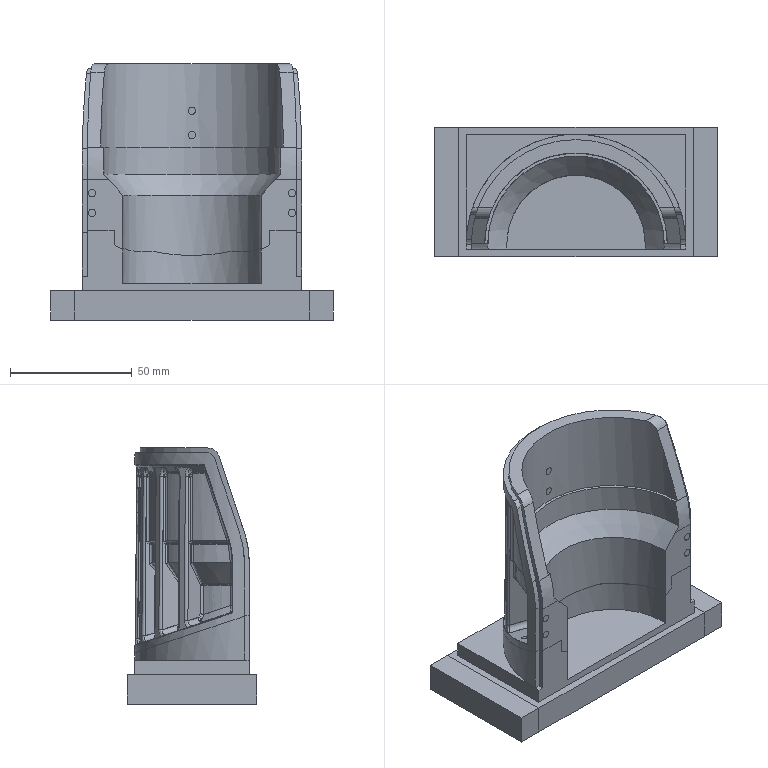NC program | NX | posted by the shop | part box 116 x 53 x 105 mm
Lines 37694 to 39157 of 44585:
T21 M6
;(T21:J-D2R0.2  D=2. R=0.2)
;(XY=0.mm Z=0.mm)
G54 G90 D1
CYCLE832(0.02,_TOP_SURFACE_SMOOTH_ON+_ORI_SEMIFIN,1.)
CYCLE800(0,"AFMING",100000,57,0.,0.,0.,-18.435,-0.,-0.,0.,0.,0.,-1,100.,1)
G0 X34.181 Y7.281 S8000 M3 M8
Z55.179
X34.181 Y7.281 Z55.179
Z-14.635
G3 X32.909 Y5.31 I.725 J-1.864 F250.
G1 X32.918 Y5.139 F2000.
X32.922 Y5.09 Z-14.652
X32.925 Y5.0406 Z-14.668
X32.9275 Y4.991 Z-14.685
X32.9062 Y5.375
X32.905 Y5.41 Z-14.735
X32.906 Y5.399
X32.937 Y4.844
X32.941 Y4.795 Z-14.752
X32.944 Y4.746 Z-14.768
X32.947 Y4.697 Z-14.785
X32.907 Y5.399
X32.904 Y5.427
X32.903 Y5.4439 Z-14.835
X32.908 Y5.399
X32.9561 Y4.55
X32.9591 Y4.5 Z-14.852
X32.961 Y4.451 Z-14.868
X32.963 Y4.401 Z-14.885
X32.957 Y4.551
X32.909 Y5.399
X32.903 Y5.461
X32.903 Y5.478 Z-14.935
X32.91 Y5.399
X32.964 Y4.41
X32.97 Y4.2525
X32.973 Y4.202 Z-14.952
X32.975 Y4.152 Z-14.968
X32.976 Y4.102 Z-14.985
G3 X32.903 Y5.495 I-39.922 J-1.395
G1 X32.904 Y5.512 Z-15.035
G2 X32.981 Y3.955 I-38.884 J-2.711
G1 X32.984 Y3.905 Z-15.052
X32.986 Y3.856 Z-15.068
X32.986 Y3.806 Z-15.085
G3 X32.905 Y5.5296 I-41.669 J-1.1077
G1 X32.905 Y5.5467 Z-15.135
G2 X32.99 Y3.655 I-40.626 J-2.775
G1 X32.992 Y3.605 Z-15.152
X32.993 Y3.556 Z-15.168
X32.993 Y3.506 Z-15.185
G3 X32.904 Y5.564 I-38.054 J-.617
G1 X32.903 Y5.581 Z-15.235
G2 X32.995 Y3.354 I-36.382 J-2.619
G1 X32.997 Y3.302 Z-15.252
X32.998 Y3.25 Z-15.268
X32.997 Y3.198 Z-15.285
G3 X32.903 Y5.5979 I-36.116 J-.216
G1 X32.903 Y5.615 Z-15.335
G2 X32.999 Y3.039 I-36.448 J-2.647
G1 X32.999 Y2.988 Z-15.352
X32.9992 Y2.936 Z-15.368
X32.999 Y2.885 Z-15.385
G3 X32.903 Y5.6322 I-36.989 J.083
G1 X32.903 Y5.649 Z-15.435
G2 X32.998 Y2.7334 I-37.618 J-2.687
G1 X32.998 Y2.677 Z-15.452
X32.998 Y2.621 Z-15.468
X32.996 Y2.565 Z-15.485
G3 X32.904 Y5.667 I-37.814 J.428
G1 X32.905 Y5.684 Z-15.535
G2 X32.994 Y2.413 I-37.856 J-2.663
G1 X32.993 Y2.361 Z-15.552
X32.993 Y2.309 Z-15.568
X32.99 Y2.257 Z-15.5849
G3 X32.904 Y5.7007 I-37.305 J.784
G1 X32.9031 Y5.718 Z-15.635
G2 X32.985 Y2.068 I-36.314 J-2.638
G1 X32.985 Y2.016 Z-15.652
X32.983 Y1.963 Z-15.668
X32.98 Y1.911 Z-15.685
G3 X32.903 Y5.735 I-36.48 J1.171
G1 X32.902 Y5.752 Z-15.735
G2 X32.975 Y1.76 I-36.482 J-2.66
G1 X32.973 Y1.69 Z-15.752
X32.97 Y1.619 Z-15.7682
X32.965 Y1.549 Z-15.785
G3 X32.9026 Y5.769 I-35.976 J1.5789
G1 X32.903 Y5.786 Z-15.835
G2 X32.959 Y1.416 I-36.41 J-2.654
G1 X32.956 Y1.3464 Z-15.852
X32.952 Y1.277 Z-15.868
X32.947 Y1.208 Z-15.885
X32.954 Y1.301
X32.9741 Y1.725
G3 X32.904 Y5.803 I-37.881 J1.386
G1 X32.905 Y5.82 Z-15.935
G2 X32.98 Y1.866 I-38.998 J-2.72
G1 X32.974 Y1.725
X32.9462 Y1.16
X32.939 Y1.068
X32.937 Y1.013 Z-15.947
X32.933 Y.958 Z-15.96
X32.929 Y.903 Z-15.972
X32.925 Y.848 Z-15.985
X32.961 Y1.442
G3 X32.904 Y5.837 I-37.871 J1.703
G1 X32.903 Y5.854 Z-16.035
G2 X32.961 Y1.442 I-37.744 J-2.705
G1 X32.918 Y.736
X32.916 Y.719
X32.9116 Y.652 Z-16.047
X32.9056 Y.5844 Z-16.0598
X32.899 Y.517 Z-16.0723
X32.894 Y.45 Z-16.0848
X32.907 Y.594
X32.954 Y1.301
X32.961 Y1.442
G3 X32.903 Y5.871 I-37.846 J1.712
G1 X32.902 Y5.888 Z-16.135
G2 X32.961 Y1.442 I-37.902 J-2.7271
X32.886 Y.336 I-24.379 J1.104
G1 X32.88 Y.268 Z-16.147
X32.873 Y.1991 Z-16.16
X32.8655 Y.131 Z-16.172
X32.859 Y.062 Z-16.185
G3 X32.961 Y1.442 I-25.175 J2.565
X32.902 Y5.905 I-38.202 J1.726
G1 X32.903 Y5.9224 Z-16.235
G2 X32.961 Y1.442 I-38.514 J-2.745
X32.848 Y-.062 I-27.6729 J1.333
G1 X32.845 Y-.111 Z-16.251
X32.839 Y-.16 Z-16.268
X32.834 Y-.2088 Z-16.285
G3 X32.961 Y1.442 I-25.577 J2.8
X32.903 Y5.939 I-39.018 J1.744
G1 X32.904 Y5.957 Z-16.335
G2 X32.968 Y1.584 I-39.836 J-2.769
X32.815 Y-.394 I-31.114 J1.412
G1 X32.808 Y-.46 Z-16.351
X32.8 Y-.526 Z-16.368
X32.791 Y-.591 Z-16.385
G3 X32.968 Y1.584 I-29.572 J3.497
X32.904 Y5.974 I-40.083 J1.611
G1 X32.903 Y5.99 Z-16.435
G2 X32.968 Y1.584 I-39.901 J-2.792
X32.769 Y-.787 I-31.046 J1.408
G1 X32.761 Y-.851 Z-16.451
X32.753 Y-.915 Z-16.468
X32.745 Y-.979 Z-16.485
G3 X32.968 Y1.584 I-30.603 J3.956
X32.903 Y6.007 I-39.963 J1.62
G1 X32.902 Y6.024 Z-16.5347
G2 X32.968 Y1.584 I-40.007 J-2.814
X32.719 Y-1.176 I-31.072 J1.41
G1 X32.712 Y-1.23 Z-16.5472
X32.705 Y-1.283 Z-16.5597
X32.697 Y-1.336 Z-16.5722
X32.69 Y-1.389 Z-16.585
G3 X32.9681 Y1.584 I-30.725 J4.377
X32.902 Y6.041 I-40.294 J1.6334
G1 X32.9024 Y6.058 Z-16.635
G2 X32.9681 Y1.584 I-40.545 J-2.833
X32.659 Y-1.6008 I-30.989 J1.403
G1 X32.651 Y-1.654 Z-16.647
X32.643 Y-1.707 Z-16.66
X32.635 Y-1.76 Z-16.672
X32.627 Y-1.813 Z-16.685
G3 X32.968 Y1.584 I-30.868 J4.815
X32.9029 Y6.075 I-41.059 J1.65
G1 X32.904 Y6.092 Z-16.735
G2 X32.974 Y1.725 I-41.896 J-2.861
X32.5932 Y-2.0265 I-31.302 J1.284
G1 X32.584 Y-2.083 Z-16.747
X32.575 Y-2.139 Z-16.76
X32.566 Y-2.1948 Z-16.772
X32.556 Y-2.251 Z-16.785
G3 X32.9742 Y1.725 I-30.923 J5.2627
X32.904 Y6.109 I-42.468 J1.515
G1 X32.903 Y6.126 Z-16.835
G2 X32.9742 Y1.725 I-42.202 J-2.881
X32.517 Y-2.478 I-31.405 J1.292
G1 X32.507 Y-2.535 Z-16.847
X32.497 Y-2.592 Z-16.86
X32.487 Y-2.648 Z-16.872
X32.476 Y-2.704 Z-16.885
G3 X32.974 Y1.725 I-30.929 J5.723
X32.9026 Y6.143 I-42.1097 J1.527
G1 X32.902 Y6.16 Z-16.935
G2 X32.974 Y1.725 I-42.084 J-2.901
X32.432 Y-2.9387 I-31.534 J1.303
G1 X32.421 Y-2.9966 Z-16.947
X32.4101 Y-3.054 Z-16.96
X32.399 Y-3.112 Z-16.972
X32.387 Y-3.17 Z-16.985
G3 X32.974 Y1.725 I-31.12 J6.213
X32.902 Y6.177 I-42.441 J1.5383
G1 X32.902 Y6.193 Z-17.035
G2 X32.974 Y1.725 I-42.602 J-2.922
X32.337 Y-3.416 I-31.689 J1.317
G1 X32.325 Y-3.477 Z-17.0471
X32.312 Y-3.538 Z-17.0596
X32.299 Y-3.5995 Z-17.0721
X32.2854 Y-3.661 Z-17.0846
G3 X32.974 Y1.725 I-31.031 J6.706
X32.903 Y6.21 I-43.098 J1.555
G1 X32.903 Y6.227 Z-17.135
G2 X32.98 Y1.866 I-44.142 J-2.958
X32.232 Y-3.909 I-31.94 J1.202
G1 X32.218 Y-3.97 Z-17.147
X32.204 Y-4.032 Z-17.16
X32.19 Y-4.094 Z-17.172
X32.176 Y-4.155 Z-17.185
G3 X32.993 Y2.349 I-30.668 J7.155
X32.904 Y6.244 I-44.932 J.929
G1 X32.904 Y6.261 Z-17.235
G2 X32.98 Y1.866 I-44.781 J-2.978
X32.116 Y-4.411 I-32.015 J1.209
G1 X32.1 Y-4.478 Z-17.247
X32.084 Y-4.5447 Z-17.26
X32.068 Y-4.611 Z-17.272
X32.0509 Y-4.678 Z-17.285
G3 X32.968 Y1.584 I-31.143 J7.76
X32.903 Y6.278 I-43.805 J1.737
G1 X32.902 Y6.294 Z-17.335
G2 X32.968 Y1.584 I-43.778 J-2.969
X31.983 Y-4.946 I-32.094 J1.503
G1 X31.969 Y-5.001 Z-17.345
X31.956 Y-5.056 Z-17.355
X31.941 Y-5.1108 Z-17.365
X31.927 Y-5.166 Z-17.375
X31.912 Y-5.221 Z-17.385
G3 X32.962 Y1.442 I-31.142 J8.322
X32.902 Y6.311 I-43.672 J1.901
G1 X32.902 Y6.3281 Z-17.435
G2 X32.962 Y1.442 I-43.9467 J-2.979
X31.838 Y-5.494 I-32.343 J1.678
G1 X31.823 Y-5.551 Z-17.445
X31.807 Y-5.608 Z-17.455
X31.791 Y-5.666 Z-17.465
X31.775 Y-5.723 Z-17.475
X31.758 Y-5.78 Z-17.485
G3 X32.962 Y1.442 I-31.17 J8.9042
X32.902 Y6.345 I-44.42 J1.915
G1 X32.903 Y6.362 Z-17.535
G2 X33. Y2.997 I-42.91 J-2.921
G1 X32.999 Y2.8974
G2 X31.81 Y-5.591 I-31.918 J.147
G1 X31.681 Y-6.047
X31.672 Y-6.076
X31.656 Y-6.135 Z-17.545
X31.6382 Y-6.194 Z-17.5545
X31.621 Y-6.253 Z-17.5645
X31.603 Y-6.3116 Z-17.5745
X31.585 Y-6.37 Z-17.5845
G3 X31.88 Y-5.341 I-30.593 J9.306
X32.9986 Y2.714 I-30.895 J8.396
G1 X33. Y2.997
G3 X32.904 Y6.379 I-43.855 J.445
G1 X32.904 Y6.396 Z-17.634
G2 X32.968 Y1.584 I-46.186 J-3.024
X31.491 Y-6.678 I-32.549 J1.559
G1 X31.471 Y-6.741 Z-17.644
X31.45 Y-6.805 Z-17.654
X31.43 Y-6.868 Z-17.664
X31.41 Y-6.932 Z-17.674
X31.389 Y-6.995 Z-17.684
G3 X32.021 Y-4.8 I-31.95 J10.38
G1 X32.053 Y-4.669
G3 X32.999 Y2.891 I-30.9 J7.706
G1 X32.9999 Y2.997
G3 X32.903 Y6.412 I-43.613 J.471
G1 X32.902 Y6.4289 Z-17.734
G2 X32.9999 Y2.997 I-43.681 J-2.959
G1 X32.999 Y2.8917
G2 X32.0531 Y-4.67 I-31.846 J.145
G1 X32.021 Y-4.8
G2 X31.287 Y-7.305 I-32.606 J8.19
G1 X31.265 Y-7.371 Z-17.744
X31.243 Y-7.437 Z-17.754
X31.221 Y-7.503 Z-17.764
X31.198 Y-7.5684 Z-17.774
X31.1754 Y-7.634 Z-17.784
G3 X31.88 Y-5.341 I-32.106 J11.118
G1 X31.955 Y-5.058
G3 X33. Y3.279 I-30.9545 J8.113
X32.902 Y6.446 I-40.668 J.3274
G1 X32.9019 Y6.462 Z-17.834
G2 X33. Y3.279 I-40.628 J-2.844
X31.955 Y-5.058 I-31.999 J-.224
G1 X31.8799 Y-5.341
G2 X31.055 Y-7.975 I-32.5408 J8.746
G1 X31.034 Y-8.033 Z-17.843
X31.013 Y-8.091 Z-17.851
X30.992 Y-8.149 Z-17.859
X30.971 Y-8.207 Z-17.868
X30.95 Y-8.264 Z-17.876
X30.9283 Y-8.322 Z-17.884
G3 X32.021 Y-4.8 I-31.77 J11.785
G1 X32.062 Y-4.634
G3 X33. Y3.138 I-30.922 J7.674
X32.902 Y6.479 I-42.146 J.438
G1 X32.903 Y6.496 Z-17.934
G2 X33. Y3.138 I-42.544 J-2.914
X32.062 Y-4.634 I-31.859 J-.099
G1 X32.021 Y-4.8
G2 X30.797 Y-8.672 I-32.9466 J8.286
G1 X30.774 Y-8.73 Z-17.943
X30.7514 Y-8.789 Z-17.951
X30.729 Y-8.848 Z-17.959
X30.706 Y-8.906 Z-17.968
X30.683 Y-8.965 Z-17.976
X30.66 Y-9.023 Z-17.984
G3 X32.815 Y-.395 I-31.093 J12.348
X33. Y3.562 I-33.052 J3.525
X32.903 Y6.513 I-40.581 J.149
G1 X32.904 Y6.53 Z-18.034
G2 X33. Y3.562 I-41.51 J-2.823
X32.815 Y-.395 I-33.238 J-.4318
X30.511 Y-9.394 I-33.279 J3.7266
G1 X30.485 Y-9.457 Z-18.043
X30.4592 Y-9.5199 Z-18.051
X30.433 Y-9.5825 Z-18.0594
X30.407 Y-9.645 Z-18.068
X30.381 Y-9.708 Z-18.076
X30.355 Y-9.7702 Z-18.0844
G3 X32.815 Y-.395 I-30.874 J13.113
X33. Y3.562 I-33.055 J3.525
X32.903 Y6.546 I-40.712 J.176
G1 X32.903 Y6.563 Z-18.134
G2 X33. Y3.562 I-40.032 J-2.801
X32.815 Y-.395 I-33.241 J-.432
X30.189 Y-10.154 I-33.366 J3.745
G1 X30.165 Y-10.211 Z-18.142
X30.14 Y-10.268 Z-18.149
X30.1141 Y-10.324 Z-18.156
X30.089 Y-10.381 Z-18.163
X30.064 Y-10.438 Z-18.1701
X30.038 Y-10.494 Z-18.177
X30.013 Y-10.551 Z-18.184
G3 X32.815 Y-.395 I-30.6103 J13.911
X33. Y3.562 I-33.058 J3.525
X32.902 Y6.58 I-39.751 J.222
G1 X32.902 Y6.596 Z-18.234
G2 X33. Y3.562 I-39.719 J-2.802
X32.815 Y-.395 I-33.244 J-.432
X30.158 Y-10.223 I-33.345 J3.741
G1 X30.042 Y-10.487
X29.824 Y-10.964
X29.795 Y-11.024 Z-18.242
X29.766 Y-11.085 Z-18.249
X29.737 Y-11.145 Z-18.2558
X29.708 Y-11.206 Z-18.263
X29.679 Y-11.266 Z-18.27
X29.6505 Y-11.327 Z-18.277
X29.622 Y-11.387 Z-18.284
G3 X30.0677 Y-10.4281 I-28.047 J13.623
X32.815 Y-.395 I-30.625 J13.78
X33. Y3.562 I-33.061 J3.525
X32.902 Y6.613 I-39.974 J.244
G1 X32.902 Y6.63 Z-18.334
G2 X33. Y3.562 I-40.344 J-2.819
X32.815 Y-.395 I-33.247 J-.432
X30.068 Y-10.4281 I-33.373 J3.746
X29.401 Y-11.834 I-30.442 J13.566
G1 X29.372 Y-11.891 Z-18.3406
X29.343 Y-11.949 Z-18.347
X29.314 Y-12.006 Z-18.3531
X29.285 Y-12.064 Z-18.359
X29.255 Y-12.121 Z-18.3656
X29.226 Y-12.178 Z-18.372
X29.196 Y-12.235 Z-18.378
X29.166 Y-12.292 Z-18.384
G3 X30.068 Y-10.4281 I-29.403 J15.3685
X32.815 Y-.395 I-30.6254 J13.779
X33. Y3.562 I-33.063 J3.525
X32.903 Y6.647 I-41.125 J.251
G1 X32.904 Y6.664 Z-18.434
G2 X33. Y3.562 I-41.947 J-2.852
X32.815 Y-.395 I-33.2495 J-.432
X30.131 Y-10.287 I-33.392 J3.75
G1 X30.068 Y-10.4281
G2 X28.92 Y-12.759 I-31.486 J14.062
G1 X28.8862 Y-12.8204 Z-18.441
X28.853 Y-12.882 Z-18.447
X28.818 Y-12.944 Z-18.453
X28.7845 Y-13.005 Z-18.459
X28.75 Y-13.067 Z-18.466
X28.716 Y-13.128 Z-18.472
X28.682 Y-13.19 Z-18.478
X28.648 Y-13.251 Z-18.484
G3 X30.068 Y-10.4281 I-29.92 J16.816
G1 X30.131 Y-10.287
G3 X32.8153 Y-.395 I-30.708 J13.642
X33. Y3.562 I-33.066 J3.525
X32.904 Y6.68 I-42.028 J.263
G1 X32.903 Y6.697 Z-18.534
G2 X33. Y3.562 I-41.332 J-2.849
X32.815 Y-.395 I-33.252 J-.431
X30.131 Y-10.287 I-33.392 J3.75
G1 X30.068 Y-10.4281
G2 X28.366 Y-13.745 I-31.535 J14.087
G1 X28.332 Y-13.802 Z-18.54
X28.299 Y-13.859 Z-18.545
X28.265 Y-13.9155 Z-18.551
X28.232 Y-13.972 Z-18.557
X28.198 Y-14.029 Z-18.562
X28.164 Y-14.085 Z-18.568
X28.13 Y-14.142 Z-18.573
X28.096 Y-14.198 Z-18.579
X28.062 Y-14.255 Z-18.5843
G3 X30.068 Y-10.4281 I-29.508 J17.904
G1 X30.131 Y-10.287
G3 X32.815 Y-.395 I-30.708 J13.642
X32.9999 Y3.562 I-33.069 J3.525
X32.9022 Y6.714 I-41.0295 J.305
G1 X32.902 Y6.73 Z-18.634
G2 X32.9999 Y3.562 I-40.7777 J-2.8472
X32.815 Y-.395 I-33.255 J-.431
X30.131 Y-10.287 I-33.392 J3.75
G1 X30.068 Y-10.4281
G2 X27.779 Y-14.713 I-31.564 J14.102
G1 X27.778 Y-14.716 Z-18.684
G3 X30.068 Y-10.4281 I-29.271 J18.388
G1 X30.131 Y-10.287
G3 X32.815 Y-.395 I-30.708 J13.642
X32.9999 Y3.562 I-33.072 J3.525
X32.902 Y6.747 I-40.9504 J.3332
G1 X32.902 Y6.764 Z-18.734
G2 X32.9999 Y3.562 I-41.176 J-2.861
X32.815 Y-.395 I-33.258 J-.431
X30.1313 Y-10.287 I-33.392 J3.75
G1 X30.068 Y-10.4281
G2 X27.776 Y-14.718 I-31.557 J14.099
G1 X27.775 Y-14.721 Z-18.784
G3 X30.0678 Y-10.4281 I-29.26 J18.389
G1 X30.131 Y-10.287
G3 X32.815 Y-.395 I-30.708 J13.642
X33. Y3.562 I-33.075 J3.526
X32.903 Y6.781 I-41.794 J.346
G1 X32.9033 Y6.797 Z-18.834
G2 X33. Y3.562 I-42.505 J-2.888
X32.815 Y-.395 I-33.261 J-.431
X30.131 Y-10.287 I-33.392 J3.75
G1 X30.068 Y-10.4281
G2 X27.7732 Y-14.723 I-31.5923 J14.1177
G1 X27.772 Y-14.726 Z-18.884
G3 X30.068 Y-10.4281 I-29.292 J18.413
G1 X30.131 Y-10.287
G3 X32.815 Y-.395 I-30.722 J13.646
X33. Y3.562 I-33.078 J3.5256
X32.904 Y6.814 I-43.446 J.347
G1 X32.903 Y6.831 Z-18.934
G2 X33. Y3.562 I-42.6791 J-2.9
X32.815 Y-.395 I-33.264 J-.431
X30.131 Y-10.287 I-33.4061 J3.754
G1 X30.068 Y-10.4281
G2 X27.77 Y-14.728 I-31.585 J14.114
G1 X27.768 Y-14.731 Z-18.984
G3 X30.068 Y-10.4281 I-29.2829 J18.415
G1 X30.131 Y-10.287
G3 X32.815 Y-.395 I-30.7221 J13.646
X33. Y3.562 I-33.08 J3.526
X32.902 Y6.847 I-42.338 J.388
G1 X32.902 Y6.8639 Z-19.034
G2 X33. Y3.562 I-41.97 J-2.897
X32.815 Y-.395 I-33.266 J-.431
X30.131 Y-10.287 I-33.406 J3.754
G1 X30.068 Y-10.4281
G2 X27.767 Y-14.733 I-31.579 J14.111
G1 X27.765 Y-14.736 Z-19.0842
G3 X30.068 Y-10.4281 I-29.231 J18.394
G1 X30.131 Y-10.287
G3 X32.815 Y-.395 I-30.708 J13.642
X33. Y3.562 I-33.0833 J3.526
X32.902 Y6.8806 I-42.132 J.4152
G1 X32.902 Y6.897 Z-19.134
G2 X33. Y3.562 I-42.3054 J-2.912
X32.815 Y-.395 I-33.269 J-.431
X30.131 Y-10.287 I-33.392 J3.75
G1 X30.068 Y-10.4281
G2 X27.764 Y-14.738 I-31.531 J14.086
G1 X27.762 Y-14.741 Z-19.184
G3 X30.068 Y-10.4281 I-29.223 J18.397
G1 X30.131 Y-10.287
G3 X32.815 Y-.395 I-30.7081 J13.642
X33. Y3.562 I-33.086 J3.526
X32.902 Y6.914 I-42.866 J.429
G1 X32.903 Y6.931 Z-19.234
G2 X33. Y3.562 I-43.544 J-2.94
X32.815 Y-.395 I-33.272 J-.431
X30.1314 Y-10.287 I-33.3921 J3.75
G1 X30.068 Y-10.4281
G2 X27.761 Y-14.743 I-31.526 J14.083
G1 X27.759 Y-14.746 Z-19.284
G3 X30.0679 Y-10.4281 I-29.258 J18.422
G1 X30.131 Y-10.287
G3 X32.815 Y-.395 I-30.708 J13.642
X33. Y3.562 I-33.089 J3.526
X32.904 Y6.948 I-44.6 J.428
G1 X32.904 Y6.9642 Z-19.334
G2 X33. Y3.562 I-44.41 J-2.961
X32.8154 Y-.395 I-33.275 J-.431
X30.131 Y-10.287 I-33.406 J3.754
G1 X30.068 Y-10.4281
G2 X27.7575 Y-14.748 I-31.564 J14.104
G1 X27.756 Y-14.7505 Z-19.384
G3 X30.068 Y-10.4281 I-29.2499 J18.425
G1 X30.131 Y-10.287
G3 X32.815 Y-.395 I-30.7222 J13.646
X33. Y3.562 I-33.0918 J3.526
X32.903 Y6.981 I-44.05 J.458
G1 X32.902 Y6.997 Z-19.434
G2 X33. Y3.562 I-43.48 J-2.957
X32.815 Y-.395 I-33.278 J-.431
X30.131 Y-10.287 I-33.406 J3.754
G1 X30.068 Y-10.4281
G2 X27.754 Y-14.753 I-31.554 J14.0984
G1 X27.753 Y-14.755 Z-19.484
G3 X30.068 Y-10.4281 I-29.236 J18.425
G1 X30.131 Y-10.287
G3 X32.815 Y-.395 I-30.722 J13.6459
X33. Y3.562 I-33.095 J3.526
X32.902 Y7.014 I-43.498 J.491
G1 X32.902 Y7.031 Z-19.534
G2 X33. Y3.562 I-43.574 J-2.968
X32.815 Y-.395 I-33.281 J-.4307
X30.131 Y-10.287 I-33.4062 J3.754
G1 X30.068 Y-10.4281
G2 X27.751 Y-14.758 I-31.549 J14.096
G1 X27.75 Y-14.76 Z-19.584
G3 X30.068 Y-10.4281 I-29.229 J18.427
G1 X30.131 Y-10.287
G3 X32.815 Y-.395 I-30.722 J13.646
X33. Y3.562 I-33.097 J3.526
X32.902 Y7.048 I-44.144 J.504
G1 X32.903 Y7.064 Z-19.6341
G2 X33. Y3.703 I-43.101 J-2.927
X32.919 Y.736 I-36.258 J-.496
X31.031 Y-8.041 I-32.955 J2.4957
G1 X30.986 Y-8.167
G2 X27.748 Y-14.763 I-32.582 J11.901
G1 X27.747 Y-14.765 Z-19.684
G3 X30.986 Y-8.167 I-29.313 J18.485
G1 X31.031 Y-8.041
G3 X32.919 Y.736 I-31.067 J11.272
X33. Y3.703 I-36.178 J2.472
X32.903 Y7.081 I-44.076 J.433
G1 X32.904 Y7.0977 Z-19.734
G2 X33. Y3.703 I-44.705 J-2.9592
X32.919 Y.736 I-36.26 J-.496
X31.088 Y-7.884 I-32.9571 J2.496
G1 X31.031 Y-8.041
G2 X27.745 Y-14.768 I-32.57 J11.745
G1 X27.743 Y-14.77 Z-19.784
G3 X31.037 Y-8.026 I-29.294 J18.481
G1 X31.088 Y-7.884
G3 X32.919 Y.736 I-31.126 J11.116
X33. Y3.703 I-36.18 J2.472
X32.903 Y7.114 I-44.497 J.446
G1 X32.902 Y7.131 Z-19.834
G2 X32.9997 Y3.703 I-44.571 J-2.981
X32.919 Y.736 I-36.263 J-.496
X31.088 Y-7.884 I-32.957 J2.496
G1 X31.037 Y-8.026
G2 X27.742 Y-14.773 I-32.587 J11.736
G1 X27.74 Y-14.7754 Z-19.884
G3 X31.037 Y-8.026 I-29.29 J18.486
G1 X31.088 Y-7.884
G3 X32.919 Y.736 I-31.126 J11.116
X32.9997 Y3.703 I-36.183 J2.472
X32.902 Y7.148 I-44.942 J.448
G1 X32.902 Y7.164 Z-19.934
G2 X33. Y3.845 I-42.236 J-2.908
X32.954 Y1.301 I-41.411 J-.533
X31.33 Y-7.178 I-32.672 J1.866
G1 X31.314 Y-7.224
G2 X27.739 Y-14.778 I-32.827 J10.916
G1 X27.737 Y-14.78 Z-19.984
G3 X31.314 Y-7.224 I-29.25 J18.471
G1 X31.33 Y-7.178
G3 X32.954 Y1.301 I-31.048 J10.345
X33. Y3.845 I-41.37 J2.011
X32.902 Y7.1809 I-42.572 J.421
G1 X32.902 Y7.198 Z-20.034
G2 X32.9998 Y3.845 I-42.85 J-2.923
X32.954 Y1.301 I-41.42 J-.533
X31.33 Y-7.178 I-32.673 J1.866
G1 X31.314 Y-7.224
G2 X27.736 Y-14.783 I-32.826 J10.915
G1 X27.734 Y-14.785 Z-20.084
G3 X31.314 Y-7.224 I-29.245 J18.475
G1 X31.33 Y-7.178
G3 X32.954 Y1.301 I-31.064 J10.348
X32.9998 Y3.845 I-41.379 J2.011
X32.903 Y7.214 I-43.4936 J.437
G1 X32.904 Y7.231 Z-20.134
G2 X32.9998 Y3.845 I-44.314 J-2.949
X32.954 Y1.301 I-41.429 J-.533
X31.33 Y-7.178 I-32.689 J1.8687
G1 X31.314 Y-7.224
G2 X27.732 Y-14.788 I-32.824 J10.914
G1 X27.731 Y-14.79 Z-20.184
G3 X31.314 Y-7.224 I-29.241 J18.48
G1 X31.33 Y-7.178
G3 X32.954 Y1.301 I-31.064 J10.3475
X33. Y3.845 I-41.388 J2.011
X32.904 Y7.246 I-44.492 J.445
G1 X32.903 Y7.261 Z-20.234
G2 X33. Y3.845 I-44.5415 J-2.97
X32.9544 Y1.301 I-41.438 J-.532
X31.3297 Y-7.178 I-32.6889 J1.869
G1 X31.314 Y-7.224
G2 X27.729 Y-14.793 I-32.823 J10.913
G1 X27.728 Y-14.795 Z-20.284
G3 X31.314 Y-7.224 I-29.256 J18.493
G1 X31.33 Y-7.178
G3 X32.9544 Y1.301 I-31.065 J10.348
X33. Y3.845 I-41.397 J2.011
X32.903 Y7.276 I-44.882 J.448
G1 X32.903 Y7.291 Z-20.334
G2 X32.999 Y4.127 I-40.367 J-2.818
X32.98 Y1.866 I-61.343 J-.613
X31.455 Y-6.79 I-32.528 J1.268
G1 X31.422 Y-6.895
G2 X27.726 Y-14.798 I-32.964 J10.601
G1 X27.725 Y-14.8 Z-20.384
G3 X31.723 Y-5.906 I-29.225 J18.485
G1 X31.738 Y-5.854
G3 X32.9928 Y2.29 I-31.014 J8.947
G1 X32.997 Y2.573
X33. Y4.496
G3 X32.903 Y7.306 I-39.05 J.056
G1 X32.903 Y7.32 Z-20.427
G2 X33. Y4.51 I-39.039 J-2.754
G1 X32.997 Y2.573
X32.9928 Y2.29
G2 X31.738 Y-5.854 I-32.268 J.802
G1 X31.7232 Y-5.906
G2 X27.723 Y-14.802 I-33.224 J9.591
G1 X27.722 Y-14.805 Z-20.469
G3 X31.723 Y-5.906 I-29.223 J18.489
X32.9928 Y2.29 I-31.031 J9.003
G1 X32.997 Y2.573
X33. Y4.524
G3 X32.903 Y7.333 I-39.302 J.056
G1 X32.904 Y7.347 Z-20.512
G2 X33. Y4.525 I-39.8023 J-2.765
G1 X32.997 Y2.573
X32.993 Y2.29
G2 X31.723 Y-5.906 I-32.3 J.807
X27.721 Y-14.8067 I-33.224 J9.591
G1 X27.72 Y-14.808 Z-20.538
G3 X31.723 Y-5.906 I-29.221 J18.493
X32.993 Y2.29 I-31.031 J9.003
G1 X32.997 Y2.573
X33. Y4.5287
G3 X32.905 Y7.355 I-40.229 J.0572
G1 X32.905 Y7.358 Z-20.546
G2 X33. Y4.5303 I-40.227 J-2.77
G1 X32.997 Y2.573
X32.993 Y2.29
G2 X31.723 Y-5.906 I-32.3 J.807
X27.72 Y-14.808 I-33.224 J9.591
G1 X27.719 Y-14.8085 Z-20.548
G3 X31.723 Y-5.906 I-29.221 J18.493
X32.993 Y2.29 I-31.031 J9.003
G1 X32.997 Y2.573
X33. Y4.523
G3 X32.905 Y7.359 I-40.567 J.058
G1 X32.905 Y7.36 Z-20.5548
G2 X33. Y4.531 I-40.331 J-2.772
G1 X32.997 Y2.573
X32.993 Y2.29
G2 X31.723 Y-5.906 I-32.3 J.807
X27.719 Y-14.8087 I-33.224 J9.591
G1 Z-19.5548
G0 Z55.179
X-34.538 Y3.281
Z-14.635
G3 X-32.918 Y5.139 I-.3775 J1.964 F250.
G1 X-32.909 Y5.31 F2000.
X-32.907 Y5.375 Z-14.685
X-32.928 Y4.992
X-32.931 Y4.9429 Z-14.702
X-32.935 Y4.894 Z-14.7184
X-32.937 Y4.845 Z-14.735
X-32.906 Y5.399
X-32.905 Y5.41
X-32.904 Y5.4268 Z-14.785
X-32.907 Y5.399
X-32.947 Y4.6972
X-32.95 Y4.648 Z-14.802
X-32.953 Y4.599 Z-14.818
X-32.956 Y4.55 Z-14.835
X-32.908 Y5.399
X-32.904 Y5.444
X-32.903 Y5.461 Z-14.885
X-32.909 Y5.399
X-32.957 Y4.551
X-32.963 Y4.402
X-32.966 Y4.353 Z-14.9017
X-32.968 Y4.303 Z-14.918
X-32.97 Y4.254 Z-14.935
X-32.964 Y4.41
X-32.91 Y5.399
X-32.903 Y5.478
X-32.904 Y5.495 Z-14.985
G3 X-32.976 Y4.103 I40.601 J-2.822
G1 X-32.979 Y4.054 Z-15.002
X-32.9805 Y4.005 Z-15.018
X-32.981 Y3.956 Z-15.035
G2 X-32.904 Y5.513 I54.042 J-1.893
G1 X-32.905 Y5.53 Z-15.085
G3 X-32.986 Y3.807 I40.932 J-2.782
G1 X-32.989 Y3.757 Z-15.102
X-32.99 Y3.707 Z-15.118
X-32.989 Y3.657 Z-15.135
G2 X-32.9052 Y5.547 I40.386 J-.853
G1 X-32.904 Y5.564 Z-15.185
G3 X-32.993 Y3.511 I37.926 J-2.66
G1 X-32.995 Y3.461 Z-15.202
X-32.996 Y3.412 Z-15.2183
X-32.995 Y3.362 Z-15.235
G2 X-32.904 Y5.581 I36.872 J-.407
G1 X-32.903 Y5.598 Z-15.285
G3 X-32.9967 Y3.208 I36.248 J-2.615
G1 X-32.999 Y3.156 Z-15.302
X-32.999 Y3.104 Z-15.318
X-32.998 Y3.053 Z-15.335
G2 X-32.903 Y5.615 I36.601 J-.076
G1 X-32.903 Y5.632 Z-15.385
G3 X-32.999 Y2.899 I36.899 J-2.654
G1 X-32.999 Y2.85 Z-15.4016
X-32.9987 Y2.8 Z-15.418
X-32.998 Y2.75 Z-15.435
G2 X-32.904 Y5.649 I37.795 J.219
G1 X-32.905 Y5.667 Z-15.485
G3 X-32.997 Y2.5911 I38.533 J-2.7
G1 X-32.996 Y2.537 Z-15.502
X-32.995 Y2.483 Z-15.518
X-32.994 Y2.429 Z-15.535
G2 X-32.905 Y5.684 I38.689 J.57
G1 X-32.904 Y5.701 Z-15.5849
G3 X-32.99 Y2.259 I37.395 J-2.657
G1 X-32.99 Y2.201 Z-15.602
X-32.988 Y2.142 Z-15.618
X-32.985 Y2.083 Z-15.635
G2 X-32.904 Y5.718 I36.608 J.998
G1 X-32.903 Y5.7348 Z-15.685
G3 X-32.979 Y1.866 I36.767 J-2.659
G1 X-32.9765 Y1.799 Z-15.71
X-32.974 Y1.732 Z-15.735
G2 X-32.9029 Y5.752 I36.613 J1.364
G1 X-32.903 Y5.769 Z-15.785
G3 X-32.969 Y1.596 I36.78 J-2.665
G1 X-32.966 Y1.526 Z-15.802
X-32.962 Y1.455 Z-15.818
X-32.956 Y1.385 Z-15.835
G2 X-32.952 Y4.937 I33.643 J1.734
G1 X-32.911 Y5.682
X-32.903 Y5.786
X-32.904 Y5.803 Z-15.885
X-32.946 Y5.068
G3 X-32.951 Y1.261 I34.3559 J-1.946
G1 X-32.948 Y1.197 Z-15.897
X-32.944 Y1.133 Z-15.91
X-32.939 Y1.069 Z-15.922
X-32.935 Y1.005 Z-15.935
G2 X-32.949 Y5.036 I34.275 J2.13
G1 X-32.905 Y5.82
X-32.904 Y5.837 Z-15.985
X-32.947 Y5.077
G3 X-32.927 Y.8685 I34.64 J-1.94
G1 X-32.923 Y.816 Z-15.997
X-32.919 Y.763 Z-16.01
X-32.915 Y.71 Z-16.022
X-32.91 Y.657 Z-16.035
G2 X-32.998 Y2.714 I27.634 J2.224
G1 X-32.999 Y2.855
G2 X-32.904 Y5.854 I39.378 J.248
G1 X-32.903 Y5.871 Z-16.0848
G3 X-32.998 Y3.562 I39.418 J-2.772
G1 X-32.999 Y3.421
G3 X-32.899 Y.513 I31.049 J-.393
G1 X-32.895 Y.45 Z-16.0973
X-32.889 Y.3876 Z-16.11
X-32.884 Y.325 Z-16.122
X-32.878 Y.262 Z-16.135
G2 X-33. Y2.997 I29.447 J2.687
G1 X-33. Y3.138
G2 X-32.903 Y5.888 I38.741 J.009
G1 X-32.903 Y5.9054 Z-16.185
G3 X-33. Y3.279 I38.606 J-2.739
G1 X-33. Y2.997
G3 X-32.8663 Y.126 I30.248 J-.031
G1 X-32.8609 Y.055 Z-16.21
X-32.853 Y-.0152 Z-16.235
G2 X-33. Y2.997 I30.346 J2.987
G1 X-33. Y3.279
G2 X-32.903 Y5.922 I39.124 J-.106
G1 X-32.904 Y5.94 Z-16.285
G3 X-33. Y3.279 I39.802 J-2.768
G1 X-33. Y2.997
G3 X-32.834 Y-.205 I30.556 J-.024
G1 X-32.828 Y-.27 Z-16.301
X-32.821 Y-.335 Z-16.318
X-32.814 Y-.401 Z-16.335
G2 X-33. Y2.997 I30.779 J3.386
G1 X-33. Y3.279
G2 X-32.905 Y5.957 I40.948 J-.114
G1 X-32.904 Y5.974 Z-16.385
G3 X-33. Y3.279 I40.742 J-2.79
G1 X-33. Y2.997
G3 X-32.792 Y-.589 I30.507 J-.027
G1 X-32.785 Y-.654 Z-16.4014
X-32.778 Y-.719 Z-16.418
X-32.77 Y-.784 Z-16.435
G2 X-33. Y2.997 I30.762 J3.77
G1 X-33. Y3.279
G2 X-32.9036 Y5.99 I39.904 J-.059
G1 X-32.903 Y6.007 Z-16.485
G3 X-33. Y3.279 I39.204 J-2.757
G1 X-33. Y2.997
G3 X-32.745 Y-.976 I30.933 J-.013
G1 X-32.7371 Y-1.041 Z-16.501
X-32.729 Y-1.107 Z-16.518
X-32.72 Y-1.173 Z-16.5347
G2 X-33. Y2.997 I30.757 J4.161
G1 X-33. Y3.279
G2 X-32.903 Y6.024 I39.0181 J-.007
G1 X-32.9026 Y6.041 Z-16.585
G3 X-33. Y2.997 I39.859 J-2.798
G1 X-32.999 Y2.855
G3 X-32.69 Y-1.389 I30.879 J.117
G1 X-32.683 Y-1.442 Z-16.597
X-32.675 Y-1.4945 Z-16.61
X-32.667 Y-1.5474 Z-16.622
X-32.659 Y-1.6 Z-16.635
G2 X-32.999 Y2.855 I30.484 J4.57
G1 X-33. Y2.997
G2 X-32.903 Y6.058 I40.272 J.256
G1 X-32.903 Y6.075 Z-16.685
G3 X-33. Y2.997 I40.788 J-2.82
G1 X-32.999 Y2.855
G3 X-32.627 Y-1.813 I31.037 J.125
G1 X-32.619 Y-1.867 Z-16.697
X-32.611 Y-1.9209 Z-16.71
X-32.602 Y-1.975 Z-16.722
X-32.593 Y-2.029 Z-16.735
G2 X-32.999 Y2.855 I30.682 J5.012
G1 X-33. Y2.997
G2 X-32.904 Y6.092 I41.765 J.2575
G1 X-32.905 Y6.109 Z-16.785
G3 X-33. Y2.997 I42.3541 J-2.853
G1 X-32.999 Y2.855
G3 X-32.556 Y-2.253 I31.154 J.131
G1 X-32.547 Y-2.31 Z-16.797
X-32.536 Y-2.367 Z-16.81
X-32.526 Y-2.424 Z-16.822
X-32.516 Y-2.481 Z-16.835
G2 X-32.999 Y2.855 I30.723 J5.47
G1 X-32.9999 Y2.997
G2 X-32.904 Y6.126 I41.666 J.286
G1 X-32.903 Y6.143 Z-16.885
G3 X-32.9999 Y2.997 I41.082 J-2.839
G1 X-32.999 Y2.855
G3 X-32.476 Y-2.705 I31.243 J.136
G1 X-32.4652 Y-2.763 Z-16.897
X-32.454 Y-2.822 Z-16.91
X-32.4432 Y-2.88 Z-16.922
X-32.432 Y-2.938 Z-16.935
G2 X-32.999 Y2.855 I30.76 J5.935
G1 X-32.9999 Y2.997
G2 X-32.903 Y6.16 I40.965 J.323
G1 X-32.902 Y6.176 Z-16.985
G3 X-32.9999 Y2.997 I41.028 J-2.848
G1 X-32.999 Y2.855
G3 X-32.388 Y-3.169 I31.443 J.1484
G1 X-32.3755 Y-3.23 Z-16.997
X-32.363 Y-3.292 Z-17.01
X-32.35 Y-3.354 Z-17.022
X-32.337 Y-3.415 Z-17.035
G2 X-32.999 Y2.714 I30.8648 J6.43
G1 X-32.9999 Y2.997
G2 X-32.9026 Y6.193 I41.335 J.342
G1 X-32.903 Y6.21 Z-17.0846
G3 X-32.9999 Y2.997 I41.719 J-2.866
G1 X-32.999 Y2.714
G3 X-32.285 Y-3.66 I31.562 J.304
G1 X-32.272 Y-3.723 Z-17.097
X-32.259 Y-3.786 Z-17.11
X-32.245 Y-3.848 Z-17.122
X-32.2312 Y-3.911 Z-17.135
G2 X-32.999 Y2.714 I30.905 J6.937
G1 X-32.9999 Y2.997
G2 X-32.904 Y6.227 I42.571 J.349
G1 X-32.905 Y6.244 Z-17.185
G3 X-32.9999 Y2.997 I43.461 J-2.899
G1 X-32.999 Y2.714
G3 X-32.176 Y-4.1542 I31.73 J.317
G1 X-32.161 Y-4.219 Z-17.197
X-32.1464 Y-4.284 Z-17.21
X-32.131 Y-4.349 Z-17.222
X-32.115 Y-4.413 Z-17.235
G2 X-32.999 Y2.714 I30.936 J7.451
G1 X-33. Y2.997
G2 X-32.904 Y6.261 I43.053 J.368
G1 X-32.903 Y6.278 Z-17.285
G3 X-33. Y2.997 I42.423 J-2.893
G1 X-32.999 Y2.714
G3 X-32.051 Y-4.68 I31.876 J.329
G1 X-32.037 Y-4.735 Z-17.295
X-32.023 Y-4.79 Z-17.305
X-32.009 Y-4.8446 Z-17.315
X-31.995 Y-4.899 Z-17.325
X-31.981 Y-4.954 Z-17.335
G2 X-32.999 Y2.8906 I30.873 J7.996
G1 X-33. Y2.997
G2 X-32.903 Y6.294 I42.243 J.405
G1 X-32.902 Y6.311 Z-17.385
G3 X-33.001 Y3.255 I41.24 J-2.862
G1 X-32.999 Y2.896
G3 X-31.908 Y-5.233 I31.947 J.151
G1 X-31.894 Y-5.289 Z-17.395
X-31.8787 Y-5.345 Z-17.405
X-31.864 Y-5.402 Z-17.415
X-31.849 Y-5.458 Z-17.425
X-31.8325 Y-5.514 Z-17.435
G2 X-32.999 Y2.714 I30.858 J8.5699
G1 X-33.0012 Y3.2712
G2 X-32.902 Y6.3281 I41.342 J.194
G1 X-32.903 Y6.345 Z-17.485
G3 X-32.984 Y2.007 I45.81 J-3.033
X-31.755 Y-5.791 I32.288 J1.092
G1 X-31.7389 Y-5.849 Z-17.495
X-31.722 Y-5.907 Z-17.505
X-31.705 Y-5.965 Z-17.515
X-31.6884 Y-6.023 Z-17.525
X-31.671 Y-6.081 Z-17.535
G2 X-32.98 Y1.866 I31.054 J9.196
X-32.903 Y6.362 I46.359 J1.457
G1 X-32.904 Y6.379 Z-17.5845
G3 X-32.974 Y1.725 I46.356 J-3.026
X-31.586 Y-6.368 I32.431 J1.399
G1 X-31.567 Y-6.43 Z-17.5945
X-31.548 Y-6.492 Z-17.604
X-31.53 Y-6.553 Z-17.614
X-31.51 Y-6.6149 Z-17.624
X-31.491 Y-6.676 Z-17.634
G2 X-32.968 Y1.584 I31.052 J9.816
X-32.9043 Y6.396 I46.3936 J1.79
G1 X-32.9034 Y6.4122 Z-17.684
G3 X-32.968 Y1.584 I46.388 J-3.0374
X-31.39 Y-6.991 I32.597 J1.566
G1 X-31.37 Y-7.054 Z-17.694
X-31.349 Y-7.1163 Z-17.704
X-31.329 Y-7.179 Z-17.714
X-31.3078 Y-7.2417 Z-17.724
X-31.287 Y-7.304 Z-17.734
G2 X-32.938 Y1.0183 I31.149 J10.503
X-33. Y3.562 I35.429 J2.137
X-32.903 Y6.429 I39.904 J.084
G1 X-32.902 Y6.446 Z-17.784
G3 X-33. Y3.562 I39.5 J-2.778
X-32.919 Y.736 I34.506 J-.421
X-31.1766 Y-7.631 I32.932 J2.492
G1 X-31.157 Y-7.688 Z-17.793
X-31.137 Y-7.744 Z-17.801
X-31.117 Y-7.801 Z-17.809
X-31.097 Y-7.857 Z-17.818
X-31.077 Y-7.914 Z-17.826
X-31.056 Y-7.97 Z-17.834
G2 X-32.919 Y.736 I31.084 J11.201
X-33. Y3.562 I34.424 J2.405
X-32.902 Y6.462 I39.558 J.122
G1 X-32.903 Y6.4793 Z-17.884
G3 X-33. Y3.562 I39.676 J-2.784
X-32.896 Y.453 I33.62 J-.435
X-30.93 Y-8.315 I32.987 J2.791
G1 X-30.909 Y-8.373 Z-17.893
X-30.888 Y-8.431 Z-17.9011
X-30.866 Y-8.489 Z-17.909
X-30.844 Y-8.547 Z-17.918
X-30.822 Y-8.605 Z-17.9261
X-30.8 Y-8.663 Z-17.934
G2 X-32.859 Y.0291 I31.088 J11.952
X-33. Y3.562 I33.262 J3.099
X-32.903 Y6.496 I40.249 J.14
G1 X-32.904 Y6.513 Z-17.984
G3 X-33. Y3.562 I40.939 J-2.811
X-32.83 Y-.254 I33.2451 J-.4327
X-30.656 Y-9.032 I33.198 J3.562
G1 X-30.632 Y-9.094 Z-17.993
X-30.607 Y-9.157 Z-18.001
X-30.582 Y-9.219 Z-18.009
X-30.557 Y-9.281 Z-18.018
X-30.532 Y-9.344 Z-18.026
X-30.506 Y-9.406 Z-18.034
G2 X-32.815 Y-.395 I30.98 J12.741
X-33. Y3.562 I33.037 J3.524
X-32.905 Y6.53 I42.061 J.137
G1 X-32.9037 Y6.546 Z-18.0844
G3 X-33. Y3.562 I41.029 J-2.816
X-32.815 Y-.395 I33.223 J-.432
X-30.348 Y-9.786 I33.342 J3.74
G1 X-30.32 Y-9.85 Z-18.093
X-30.2927 Y-9.915 Z-18.101
X-30.265 Y-9.9798 Z-18.1094
X-30.237 Y-10.045 Z-18.118
X-30.209 Y-10.109 Z-18.126
X-30.181 Y-10.173 Z-18.134
G2 X-32.815 Y-.395 I30.755 J13.529
X-33. Y3.562 I33.04 J3.524
X-32.903 Y6.563 I40.51 J.194
G1 X-32.902 Y6.5798 Z-18.184
G3 X-32.99 Y4.654 I36.454 J-2.6192
X-32.994 Y2.447 I64.185 J-1.218
X-32.669 Y-1.539 I30.341 J.467
X-30.005 Y-10.57 I33.471 J4.966
G1 X-29.978 Y-10.629 Z-18.192
X-29.951 Y-10.6878 Z-18.199
X-29.924 Y-10.747 Z-18.2058
X-29.897 Y-10.806 Z-18.213
X-29.87 Y-10.865 Z-18.22
X-29.842 Y-10.924 Z-18.227
X-29.814 Y-10.982 Z-18.234
G2 X-32.67 Y-1.533 I30.6533 J14.419
X-32.992 Y2.369 I29.907 J4.435
X-32.986 Y4.845 I61.4832 J1.083
X-32.902 Y6.597 I35.011 J-.793
G1 X-32.902 Y6.613 Z-18.284
G3 X-32.99 Y4.6731 I35.931 J-2.598
X-32.995 Y2.479 I67.517 J-1.233
X-32.671 Y-1.525 I30.264 J.431
X-29.612 Y-11.406 I33.54 J4.969
G1 X-29.5819 Y-11.468 Z-18.2915
X-29.551 Y-11.531 Z-18.299
X-29.521 Y-11.5936 Z-18.306
X-29.49 Y-11.656 Z-18.313
X-29.459 Y-11.719 Z-18.32
X-29.428 Y-11.781 Z-18.327
X-29.397 Y-11.843 Z-18.334
G2 X-32.608 Y-1.937 I30.384 J15.3226
X-32.993 Y2.434 I30.152 J4.861
X-32.987 Y4.805 I63.936 J1.026
X-32.903 Y6.63 I36.004 J-.757
G1 X-32.903 Y6.647 Z-18.384
G3 X-32.992 Y4.576 I38.152 J-2.678
X-32.996 Y2.549 I71.288 J-1.1307
X-32.607 Y-1.946 I30.591 J.384
X-29.166 Y-12.294 I33.611 J5.43
G1 X-29.135 Y-12.352 Z-18.391
X-29.105 Y-12.41 Z-18.397
X-29.074 Y-12.468 Z-18.403
X-29.0429 Y-12.526 Z-18.409
X-29.012 Y-12.585 Z-18.416
X-28.981 Y-12.643 Z-18.422
X-28.951 Y-12.701 Z-18.428
X-28.92 Y-12.759 Z-18.434
G2 X-32.5615 Y-2.222 I30.036 J16.28
X-32.994 Y2.469 I30.208 J5.151
X-32.991 Y4.682 I66.5576 J.999
X-32.904 Y6.664 I39.232 J-.715
G1 X-32.904 Y6.68 Z-18.484
G3 X-32.99 Y4.74 I37.888 J-2.644
X-32.995 Y2.5015 I68.7342 J-1.274
X-32.56 Y-2.228 I30.656 J.43
X-28.652 Y-13.242 I33.68 J5.75
G1 X-28.6212 Y-13.298 Z-18.49
X-28.59 Y-13.3535 Z-18.495
X-28.559 Y-13.409 Z-18.501
X-28.527 Y-13.464 Z-18.507
X-28.495 Y-13.519 Z-18.512
X-28.464 Y-13.5745 Z-18.518
X-28.432 Y-13.63 Z-18.5232
X-28.4001 Y-13.685 Z-18.529
X-28.3682 Y-13.74 Z-18.534
G2 X-32.375 Y-3.232 I29.648 J17.324
X-32.997 Y2.641 I30.713 J6.2208
X-32.9902 Y4.726 I72.505 J.803
X-32.903 Y6.697 I37.339 J-.66
G1 X-32.903 Y6.714 Z-18.5843
G3 X-32.99 Y4.744 I36.494 J-2.61
X-32.997 Y2.6396 I73.7531 J-1.291
X-32.377 Y-3.223 I31.3041 J.345
X-28.0618 Y-14.255 I33.673 J6.813
G1 X-28.0255 Y-14.314 Z-18.59
X-27.989 Y-14.374 Z-18.595
X-27.953 Y-14.434 Z-18.601
X-27.916 Y-14.493 Z-18.607
X-27.879 Y-14.552 Z-18.612
X-27.842 Y-14.612 Z-18.618
X-27.805 Y-14.671 Z-18.623
X-27.768 Y-14.73 Z-18.629
X-27.731 Y-14.789 Z-18.634
G2 X-32.378 Y-3.219 I29.045 J18.385
X-32.997 Y2.658 I30.646 J6.199
X-32.994 Y4.577 I80.353 J.825
X-32.902 Y6.73 I37.371 J-.509
G1 X-32.902 Y6.747 Z-18.684
G3 X-32.994 Y4.57 I37.388 J-2.668
X-32.997 Y2.66 I82.007 J-1.0747
X-32.379 Y-3.216 I31.258 J.3181
X-27.627 Y-14.953 I33.693 J6.812
G1 X-27.624 Y-14.956 Z-18.734
G2 X-32.379 Y-3.216 I28.939 J18.552
X-32.997 Y2.663 I30.637 J6.194
X-32.995 Y4.553 I83.737 J.844
X-32.9025 Y6.764 I37.91 J-.474
G1 X-32.903 Y6.78 Z-18.784
G3 X-32.995 Y4.526 I38.139 J-2.684
X-32.999 Y2.783 I97.927 J-1.099
X-32.378 Y-3.219 I31.3131 J.206
X-27.622 Y-14.96 I33.693 J6.8148
G1 X-27.619 Y-14.964 Z-18.834
G2 X-32.378 Y-3.22 I28.935 J18.56
X-32.999 Y2.789 I30.691 J6.209
X-32.996 Y4.477 I101.328 J.646
X-32.904 Y6.797 I39.645 J-.408
G1 X-32.905 Y6.814 Z-18.884
G3 X-32.996 Y4.448 I40.575 J-2.756
X-32.999 Y2.794 I104.897 J-1.004
X-32.378 Y-3.219 I31.309 J.194
X-27.6171 Y-14.968 I33.694 J6.815
G1 X-27.615 Y-14.971 Z-18.934
G2 X-32.378 Y-3.221 I28.931 J18.567
X-32.997 Y2.573 I31.014 J6.247
G1 X-32.999 Y2.714
X-32.996 Y4.551
X-32.995 Y4.625
G2 X-32.904 Y6.831 I41.5807 J-.625
G1 X-32.903 Y6.847 Z-18.984
G3 X-32.994 Y4.692 I40.106 J-2.78
G1 X-32.999 Y4.41
X-32.999 Y2.714
X-32.997 Y2.573
G3 X-32.378 Y-3.221 I31.634 J.453
X-27.612 Y-14.975 I33.694 J6.817
G1 X-27.61 Y-14.979 Z-19.034
G2 X-32.378 Y-3.221 I28.927 J18.575
X-32.997 Y2.573 I31.014 J6.247
G1 X-32.999 Y2.714
X-32.999 Y4.41
X-32.995 Y4.692
G2 X-32.902 Y6.864 I39.698 J-.597
G1 X-32.902 Y6.881 Z-19.0842
G3 X-32.995 Y4.692 I39.61 J-2.773
G1 X-32.999 Y4.41
X-32.999 Y2.714
X-32.997 Y2.573
G3 X-32.378 Y-3.221 I31.634 J.4533
X-27.608 Y-14.982 I33.695 J6.818
G1 X-27.605 Y-14.986 Z-19.134
G2 X-32.3777 Y-3.221 I28.922 J18.583
X-32.997 Y2.573 I31.015 J6.247
G1 X-32.999 Y2.714
X-32.999 Y4.41
X-32.995 Y4.692
G2 X-32.902 Y6.897 I40.074 J-.583
G1 X-32.903 Y6.914 Z-19.184
G3 X-32.995 Y4.692 I40.783 J-2.816
G1 X-32.9992 Y4.41
X-32.999 Y2.714
X-32.997 Y2.573
G3 X-32.378 Y-3.221 I31.634 J.453
X-27.603 Y-14.9898 I33.695 J6.818
G1 X-27.601 Y-14.994 Z-19.234
G2 X-32.378 Y-3.221 I28.919 J18.59
X-32.997 Y2.573 I31.015 J6.247
G1 X-32.999 Y2.714
X-32.999 Y4.41
X-32.996 Y4.692
G2 X-32.903 Y6.931 I42.173 J-.62
G1 X-32.904 Y6.948 Z-19.284
G3 X-32.996 Y4.692 I44.019 J-2.922
G1 X-32.999 Y4.41
X-32.999 Y2.714
X-32.997 Y2.573
G3 X-32.378 Y-3.221 I31.634 J.453
X-27.598 Y-14.997 I33.696 J6.818
G1 X-27.5959 Y-15.001 Z-19.334
G2 X-32.378 Y-3.221 I28.9146 J18.598
X-32.997 Y2.573 I31.015 J6.247
G1 X-32.999 Y2.714
X-32.999 Y4.41
X-32.996 Y4.692
G2 X-32.904 Y6.964 I43.724 J-.641
G1 X-32.903 Y6.981 Z-19.384
G3 X-32.996 Y4.75 I42.101 J-2.8668
G1 X-32.999 Y4.551
X-32.999 Y2.714
X-32.997 Y2.573
G3 X-32.378 Y-3.221 I31.634 J.453
X-27.594 Y-15.005 I33.697 J6.8182
G1 X-27.591 Y-15.008 Z-19.434
G2 X-32.378 Y-3.221 I28.911 J18.606
X-32.9974 Y2.573 I31.015 J6.247
G1 X-32.999 Y2.714
X-32.999 Y4.551
X-32.994 Y4.834
G2 X-32.903 Y6.997 I40.383 J-.627
G1 X-32.902 Y7.0141 Z-19.484
G3 X-32.995 Y4.834 I39.83 J-2.778
G1 X-32.999 Y4.551
X-32.999 Y2.714
X-32.9974 Y2.573
G3 X-32.378 Y-3.221 I31.634 J.453
X-27.589 Y-15.012 I33.698 J6.818
G1 X-27.586 Y-15.016 Z-19.534
G2 X-32.378 Y-3.221 I28.907 J18.613
X-32.997 Y2.573 I31.015 J6.247
G1 X-32.999 Y2.714
X-32.999 Y4.551
X-32.9959 Y4.786
G2 X-32.902 Y7.031 I40.629 J-.57
G1 X-32.902 Y7.048 Z-19.584
G3 X-32.995 Y4.834 I40.3203 J-2.798
G1 X-32.9992 Y4.551
X-32.999 Y2.714
X-32.997 Y2.573
G3 X-32.378 Y-3.221 I31.634 J.453
X-27.584 Y-15.019 I33.699 J6.819
G1 X-27.582 Y-15.023 Z-19.6341
G2 X-32.378 Y-3.221 I28.903 J18.621
X-32.997 Y2.573 I31.015 J6.247
G1 X-32.9988 Y2.714
X-32.999 Y4.551
G2 X-32.903 Y7.0643 I40.181 J-.28
G1 X-32.9038 Y7.081 Z-19.684
G3 X-32.999 Y4.692 I44.201 J-2.949
G1 X-32.999 Y4.551
X-32.9988 Y2.714
X-32.997 Y2.573
G3 X-32.378 Y-3.221 I31.634 J.453
X-27.579 Y-15.027 I33.696 J6.8174
G1 X-27.577 Y-15.031 Z-19.734
G2 X-32.378 Y-3.221 I28.896 J18.627
X-32.997 Y2.573 I31.015 J6.247
G1 X-32.999 Y2.714
X-32.999 Y4.304
G2 X-32.904 Y7.098 I41.489 J-.002
G1 X-32.903 Y7.114 Z-19.784
G3 X-32.999 Y4.333 I40.565 J-2.782
G1 X-32.999 Y2.714
X-32.997 Y2.573
G3 X-32.378 Y-3.221 I31.634 J.453
X-27.575 Y-15.034 I33.697 J6.818
G1 X-27.572 Y-15.038 Z-19.834
G2 X-32.3778 Y-3.221 I28.892 J18.635
X-32.997 Y2.573 I31.015 J6.247
G1 X-32.999 Y2.714
X-32.999 Y4.358
G2 X-32.903 Y7.131 I40.044 J.001
G1 X-32.902 Y7.148 Z-19.884
G3 X-32.9951 Y4.975 I40.715 J-2.827
G1 X-32.999 Y4.692
X-32.999 Y2.714
X-32.997 Y2.573
G3 X-32.3778 Y-3.221 I31.6344 J.453
X-27.57 Y-15.042 I33.695 J6.817
G1 X-27.568 Y-15.045 Z-19.934
G2 X-32.378 Y-3.221 I28.885 J18.641
X-32.997 Y2.573 I31.015 J6.247
G1 X-32.999 Y2.714
X-32.999 Y4.692
X-32.995 Y4.975
G2 X-32.902 Y7.164 I40.397 J-.623
G1 X-32.902 Y7.181 Z-19.984
G3 X-32.998 Y4.834 I40.887 J-2.84
G1 X-32.999 Y4.692
X-32.999 Y2.714
X-32.997 Y2.573
G3 X-32.378 Y-3.221 I31.634 J.453
X-27.565 Y-15.049 I33.696 J6.817
G1 X-27.563 Y-15.053 Z-20.034
G2 X-32.378 Y-3.221 I28.882 J18.649
X-32.997 Y2.573 I31.015 J6.247
G1 X-32.999 Y2.714
X-32.999 Y4.4347
G2 X-32.903 Y7.198 I39.608 J.003
G1 X-32.903 Y7.2144 Z-20.084
G3 X-32.999 Y4.48 I40.046 J-2.767
G1 X-33. Y2.997
X-32.999 Y2.797
G3 X-32.383 Y-3.197 I31.274 J.186
X-27.561 Y-15.057 I33.702 J6.793
G1 X-27.5582 Y-15.06 Z-20.134
G2 X-32.38 Y-3.21 I28.879 J18.657
X-32.999 Y2.862 I30.685 J6.198
G1 X-33. Y2.997
X-32.999 Y4.551
G2 X-32.904 Y7.231 I40.191 J-.084
G1 X-32.904 Y7.246 Z-20.184
G3 X-32.9993 Y4.551 I40.099 J-2.767
G1 X-33. Y2.997
X-32.999 Y2.862
G3 X-32.38 Y-3.21 I31.303 J.125
X-27.556 Y-15.064 I33.7011 J6.807
G1 X-27.553 Y-15.068 Z-20.234
G2 X-32.383 Y-3.196 I28.8752 J18.665
X-32.999 Y2.798 I30.656 J6.179
G1 X-33. Y2.997
X-32.999 Y4.834
X-32.997 Y4.975
G2 X-32.903 Y7.261 I41.2835 J-.545
G1 X-32.903 Y7.276 Z-20.284
G3 X-32.995 Y5.116 I39.465 J-2.76
G1 X-32.999 Y4.834
X-33. Y2.997
X-32.999 Y2.7977
G3 X-32.383 Y-3.196 I31.271 J.185
X-27.551 Y-15.071 I33.705 J6.794
G1 X-27.549 Y-15.075 Z-20.334
G2 X-32.323 Y-3.489 I28.897 J18.684
X-32.999 Y2.814 I30.779 J6.488
G1 X-33. Y2.997
X-32.999 Y4.834
X-32.995 Y5.116
G2 X-32.903 Y7.291 I38.977 J-.5649
G1 X-32.9029 Y7.306 Z-20.384
G3 X-32.998 Y4.975 I39.497 J-2.7747
G1 X-32.999 Y4.834
X-33. Y2.997
X-32.999 Y2.8138
G3 X-32.323 Y-3.487 I31.452 J.185
X-27.546 Y-15.079 I33.673 J7.097
G1 X-27.544 Y-15.082 Z-20.427
G2 X-32.323 Y-3.487 I28.8949 J18.692
X-32.999 Y2.814 I30.775 J6.486
G1 X-33. Y2.997
X-32.999 Y4.834
X-32.998 Y4.975
G2 X-32.903 Y7.32 I39.726 J-.432
G1 X-32.904 Y7.333 Z-20.469
G3 X-32.998 Y4.975 I39.685 J-2.773
G1 X-32.999 Y4.834
X-33. Y2.997
X-32.999 Y2.814
G3 X-32.323 Y-3.488 I31.4498 J.185
X-27.5424 Y-15.085 I33.675 J7.0977
G1 X-27.54 Y-15.088 Z-20.512
G2 X-32.323 Y-3.487 I28.893 J18.6988
X-32.999 Y2.814 I30.772 J6.485
G1 X-33. Y2.997
X-32.999 Y4.663
G2 X-32.904 Y7.347 I39.022 J-.03
G1 X-32.9047 Y7.355 Z-20.538
G3 X-32.999 Y4.975 I41.201 J-2.8195
G1 X-32.999 Y4.834
X-33. Y2.997
X-33. Y2.879
G3 X-32.321 Y-3.499 I31.472 J.123
X-27.539 Y-15.09 I33.6741 J7.11
G1 X-27.5388 Y-15.091 Z-20.546
G2 X-32.321 Y-3.499 I28.892 J18.702
X-33. Y2.879 I30.793 J6.501
G1 X-33. Y2.997
X-32.999 Y4.834
X-32.9988 Y4.975
G2 X-32.905 Y7.358 I41.766 J-.453
G1 X-32.905 Y7.359 Z-20.548
G3 X-32.999 Y4.975 I41.963 J-2.8469
G1 X-32.999 Y4.834
X-33. Y2.997
X-33. Y2.879
G3 X-32.321 Y-3.499 I31.472 J.123
X-27.539 Y-15.091 I33.674 J7.11
G1 X-27.538 Y-15.091 Z-20.5548
G2 X-32.321 Y-3.499 I28.892 J18.702
X-33. Y2.879 I30.793 J6.501
G1 X-33. Y2.997
X-32.999 Y4.834
X-32.999 Y4.975
G2 X-32.905 Y7.36 I42.252 J-.468
G1 Z-19.5548
G0 Z55.179
X16.531 Y-24.434
Z-20.5548
G3 X14.536 Y-22.4333 I-2. J.001 F250.
G2 X14.0039 Y-22.242 I.002 J.84 F2000.
G1 X13.939 Y-22.184
X13.895 Y-22.136
X13.857 Y-22.0891
X13.821 Y-22.035
X13.808 Y-22.014
X13.796 Y-21.993
X13.78 Y-21.961
X13.765 Y-21.931
X13.74 Y-21.866
X13.7172 Y-21.784
X13.699 Y-21.687
X13.696 Y-21.542
G2 X13.873 Y-21.057 I.819 J-.025
G1 Z-19.5548
G0 Z-17.548
X-13.582 Y-18.4069
Z-20.5548
G3 X-13.873 Y-21.057 I1.337 J-1.488 F250.
G2 X-13.696 Y-21.542 I-.475 J-.449 F2000.
G1 X-13.699 Y-21.687
X-13.717 Y-21.784
X-13.729 Y-21.849
X-13.756 Y-21.909
X-13.765 Y-21.929
X-13.78 Y-21.9623
X-13.796 Y-21.993
X-13.808 Y-22.014
X-13.832 Y-22.0504
X-13.832 Y-22.05
X-13.843 Y-22.067
X-13.861 Y-22.093
X-13.893 Y-22.1341
X-13.939 Y-22.184
X-14.0039 Y-22.242
G2 X-14.536 Y-22.4333 I-.537 J.657
G1 Z-19.5548
G0 Z55.179
CYCLE800()
CYCLE832()
;(T21:J-D2R0.2  D=2. R=0.2)
;(XY=-0.02mm Z=-0.02mm)
G54 G90 D1
CYCLE832(0.04,_TOP_SURFACE_SMOOTH_ON+_ORI_SEMIFIN,1.)
TRAFOOF
CYCLE800(0,"AFMING",100000,57,0.,0.,0.,-18.435,-0.,-0.,0.,0.,0.,-1,100.,1)
G0 X-30.162 Y-25.418 S8000 M3
Z55.179
X-30.162 Y-25.418 Z55.179
Z-19.5548
G3 X-29.877 Y-25.418 I.142 J0.0 F600.
X-29.877 Y-25.418 Z-24.5548 I-.2845 J0.0 TURN=99
X-29.877 Y-25.418 I-.2845 J0.0
X-30.162 Y-25.418 I-.142 J0.0
G0 Z55.179
X-40.223 Y-6.034
Z-19.5548
G3 X-39.939 Y-6.034 I.142 J0.0
X-39.939 Y-6.034 Z-24.5548 I-.2845 J0.0 TURN=99
X-39.939 Y-6.034 I-.2845 J0.0
X-40.223 Y-6.034 I-.142 J0.0
G0 Z55.179
X40.223
Z-19.5548
G3 X40.508 Y-6.034 I.142 J0.0
X40.508 Y-6.034 Z-24.5548 I-.2845 J0.0 TURN=99
X40.508 Y-6.034 I-.2845 J0.0
X40.223 Y-6.034 I-.142 J0.0
G0 Z55.179
X30.162 Y-25.418
Z-19.5548
G3 X30.446 Y-25.418 I.142 J0.0
X30.446 Y-25.418 Z-24.5548 I-.2845 J0.0 TURN=99
X30.446 Y-25.418 I-.2845 J0.0
X30.162 Y-25.418 I-.142 J0.0
G0 Z55.179
CYCLE800()
M9
M5
M01
TRAFOOF
SUPA G0 Z-1. D0
SUPA G0 X-1.0 Y-1.0